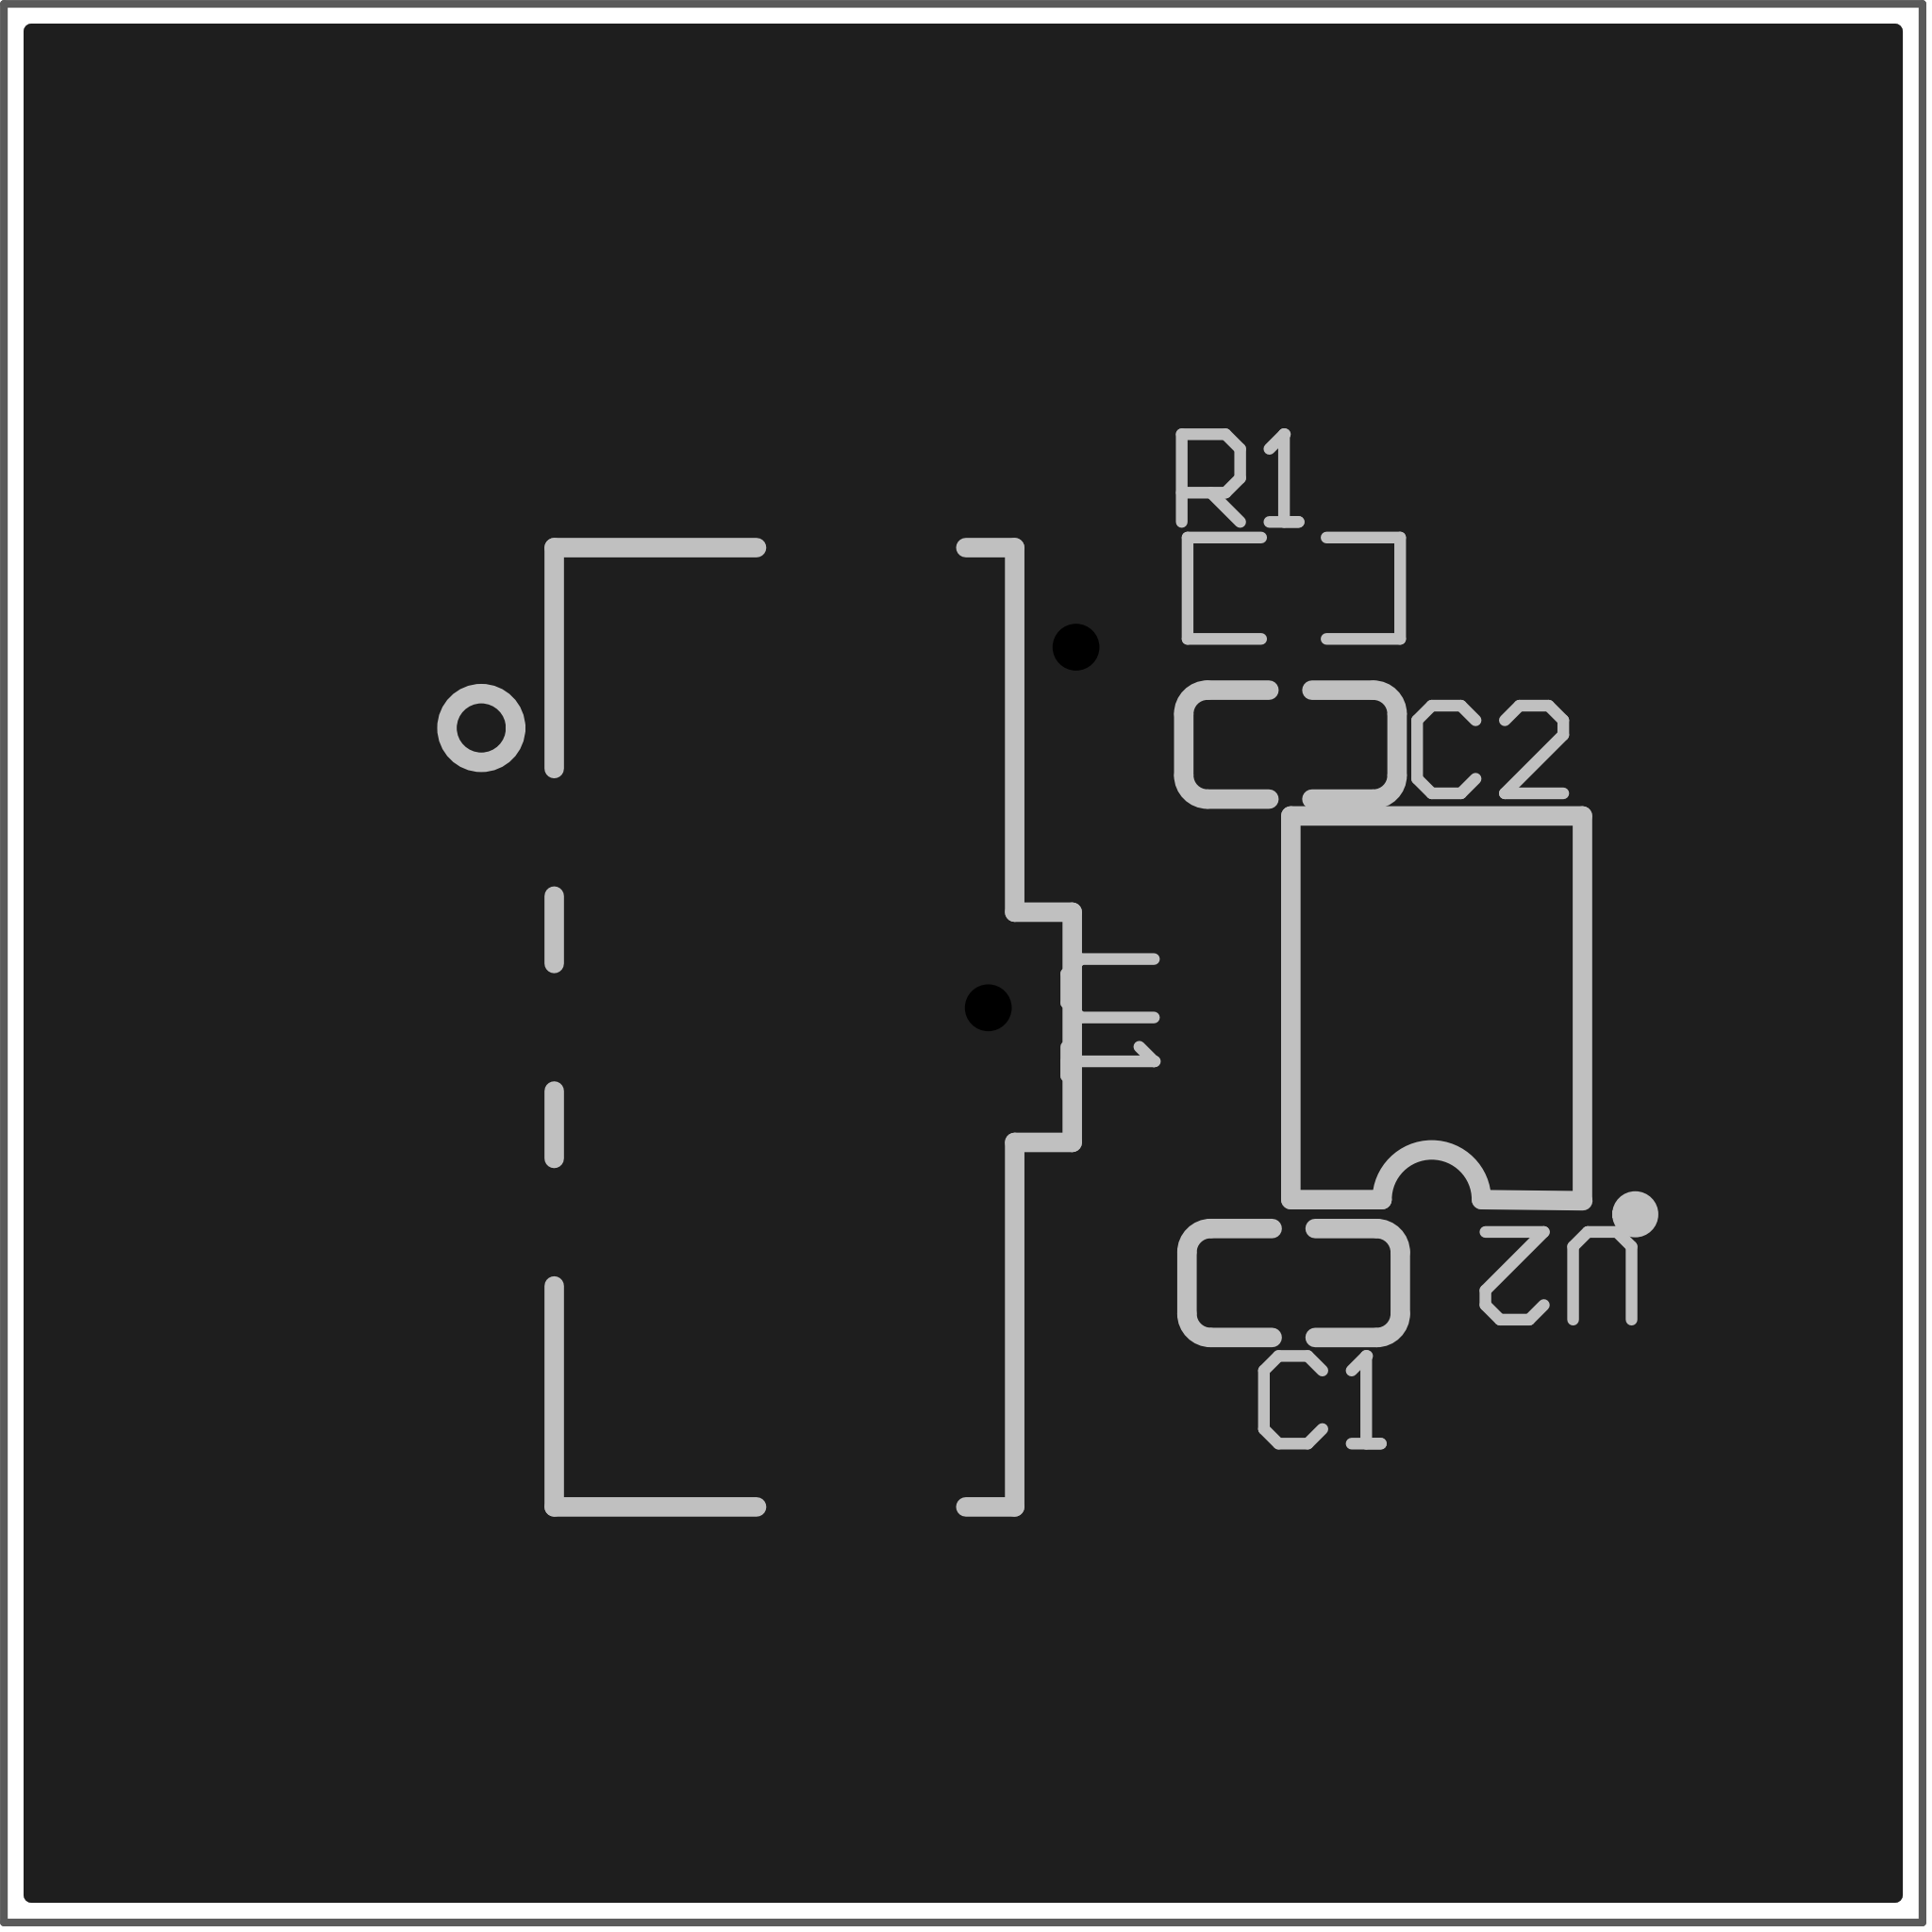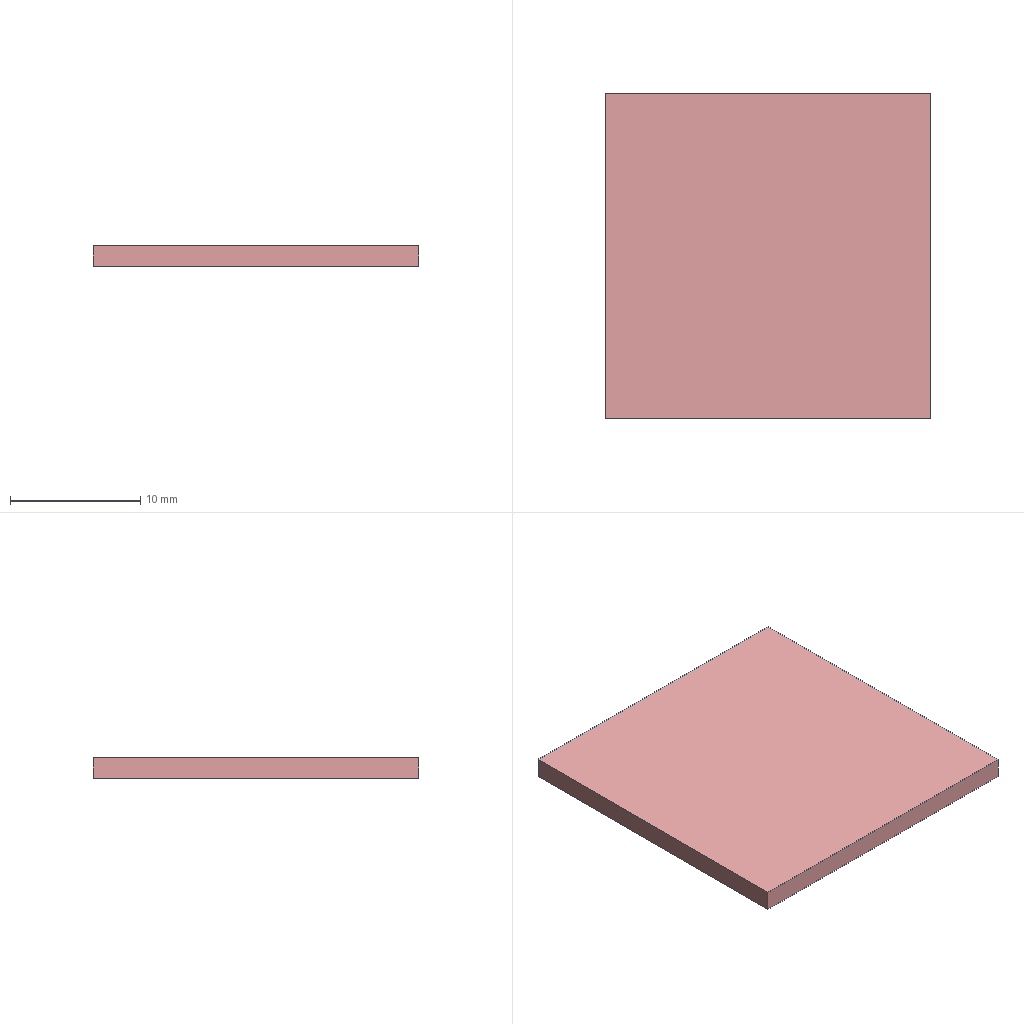Circuit board layout | Altium Designer | box 25 x 25 x 1.6 mm
Layer stack:
# Altium Designer layer stack of  (unit mm; dielectric type: 0 none, 1 core, 2 prepreg, 3 surface material)
index,name,kind,layer,copper_thickness_mm,dielectric_type,dielectric_thickness_mm,dielectric_material,dielectric_constant
0,Top Paste Mask Layer,other,,,,,,
1,Top Silkscreen Layer,other,,,,,,
2,Top Solder Mask Layer,dielectric,,,3,0.01,,3.3
3,Top Layer,copper,Top Layer,0.035,,,,
4,Dielectric1,dielectric,,,3,1.51,FR4,4.5
5,Bottom Layer,copper,Bottom Layer,0.035,,,,
6,Bottom Solder Mask Layer,dielectric,,,3,0.01,,3.3
7,Bottom Silkscreen Layer,other,,,,,,
8,Bottom Paste Mask Layer,other,,,,,,
# drill layer pairs: low layer,high layer
drill_pair,Top Layer,Bottom Layer
Part placement:
Designator,Comment,Layer,Footprint,Center-X(mm),Center-Y(mm),Rotation
C1,100nF,TopLayer,C0603,98.594,88.234,180
C2,10uF,TopLayer,C0603,98.552,95.25,0
LED1,,BottomLayer,LED_0603,92.634,91.813,180
R1,100,TopLayer,R0603,98.597,97.288,0
U1,2.543PIN vertical latching terminal,TopLayer,CONN-SMD_3P-P2.54_C9900012759,91.059,91.567,90
U2,ATW62D,TopLayer,SOP-8_L4.9-W3.9-P1.27-LS6.0-TL,100.457,91.821,180
Pad and via stacks:
# Altium Designer via and pad stacks of  (unit mm). Each distinct definition once, with the count of objects using it.
# via: kind,start_layer,end_layer,hole_mm,diameter_mm,mode(0 simple;1 top-mid-bottom;2 full stack),diameter_per_layer,count,example_net
# pad: kind,layer,hole_mm,hole_type(0 round;1 square;2 slot),plating,top_size,top_shape(1 round;2 rect;3 octagon;9 rounded rect),mid_size,bottom_size,mode,footprint,size_per_layer,count,example
pad,Top Layer,0,0,plated,0.8x0.9,2,0.8x0.9,0.8x0.9,0,C0603,,4,C1.2
pad,Top Layer,0,0,plated,0.8065x0.864,2,0.8065x0.864,0.8065x0.864,0,R0603,,2,R1.2
pad,Top Layer,0,0,plated,1.1x2.5,2,1.1x2.5,1.1x2.5,0,CONN-SMD_3P-P2.54_C9900012759,,2,U1.5
pad,Top Layer,0,0,plated,1.2x6,2,1.2x6,1.2x6,0,CONN-SMD_3P-P2.54_C9900012759,,3,U1.3
pad,Top Layer,0,0,plated,0.6x1.6,1,0.6x1.6,0.6x1.6,0,SOP-8_L4.9-W3.9-P1.27-LS6.0-TL,,8,U2.5
pad,Bottom Layer,0,0,plated,0.8001x0.8001,2,0.8001x0.8001,0.8001x0.8001,0,LED_0603,,2,LED1.1
via,Top Layer,Bottom Layer,0.3048,0.61,0,,2,$1N7
Copper pours:
name,layer,net,type(0 solid;1 hatched;2 none)
Top Layer-GND,Top Layer,GND,0
Bottom Layer-GND,Bottom Layer,GND,0